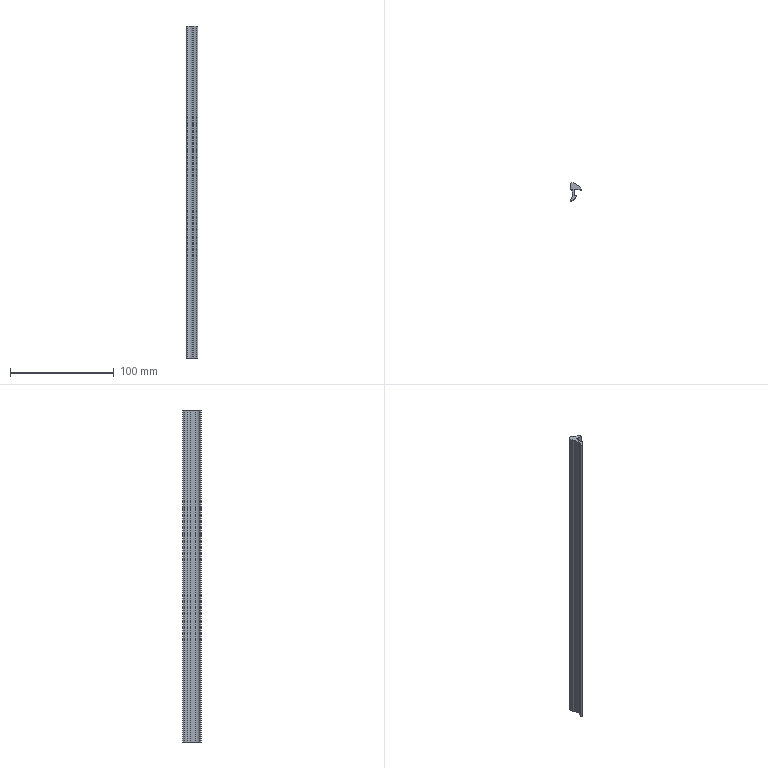Part | SolidWorks | features BaseBody 1, MoveFace 1 | 1 solid | 20 faces | box 10.8 x 17.5 x 320 mm | volume 25216 mm3 | cylinder 11 | plane 9 | commonest cylinder face diameters 1.6 x2 14 x2 0.4 x1 0.6 x1 0.8 x1 2.6 x1
STEP:
#1=CARTESIAN_POINT('',(-3.236,-11.055,220.));
#2=VERTEX_POINT('',#1);
#3=CARTESIAN_POINT('',(-4.3,-10.3,220.));
#4=VERTEX_POINT('',#3);
#5=CARTESIAN_POINT('',(-3.5,-10.3,220.));
#6=DIRECTION('',(0.,0.,-1.));
#7=DIRECTION('',(1.,0.,0.));
#8=AXIS2_PLACEMENT_3D('',#5,#6,#7);
#9=CIRCLE('',#8,0.8);
#10=EDGE_CURVE('',#2,#4,#9,.T.);
#11=ORIENTED_EDGE('',*,*,#10,.T.);
#12=CARTESIAN_POINT('',(-4.3,-10.3,-100.));
#13=VERTEX_POINT('',#12);
#14=CARTESIAN_POINT('',(-4.3,-10.3,-100.));
#15=DIRECTION('',(0.,0.,-1.));
#16=VECTOR('',#15,1000.);
#17=LINE('',#14,#16);
#18=EDGE_CURVE('',#4,#13,#17,.T.);
#19=ORIENTED_EDGE('',*,*,#18,.T.);
#20=CARTESIAN_POINT('',(-3.236,-11.055,-100.));
#21=VERTEX_POINT('',#20);
#22=CARTESIAN_POINT('',(-3.5,-10.3,-100.));
#23=DIRECTION('',(0.,0.,1.));
#24=DIRECTION('',(-1.,0.,0.));
#25=AXIS2_PLACEMENT_3D('',#22,#23,#24);
#26=CIRCLE('',#25,0.8);
#27=EDGE_CURVE('',#13,#21,#26,.T.);
#28=ORIENTED_EDGE('',*,*,#27,.T.);
#29=CARTESIAN_POINT('',(-3.236,-11.055,-100.));
#30=DIRECTION('',(0.,0.,-1.));
#31=VECTOR('',#30,1000.);
#32=LINE('',#29,#31);
#33=EDGE_CURVE('',#2,#21,#32,.T.);
#34=ORIENTED_EDGE('',*,*,#33,.F.);
#35=EDGE_LOOP('',(#11,#19,#28,#34));
#36=FACE_OUTER_BOUND('',#35,.T.);
#37=CARTESIAN_POINT('',(-3.5,-10.3,-100.));
#38=DIRECTION('',(0.,0.,-1.));
#39=DIRECTION('',(-1.,0.,0.));
#40=AXIS2_PLACEMENT_3D('',#37,#38,#39);
#41=CYLINDRICAL_SURFACE('',#40,0.8);
#42=ADVANCED_FACE('',(#36),#41,.T.);
#43=CARTESIAN_POINT('',(1.184,-6.397,-100.));
#44=VERTEX_POINT('',#43);
#45=CARTESIAN_POINT('',(-5.702,-4.29,-100.));
#46=DIRECTION('',(0.,0.,1.));
#47=DIRECTION('',(-1.,0.,0.));
#48=AXIS2_PLACEMENT_3D('',#45,#46,#47);
#49=CIRCLE('',#48,7.201);
#50=EDGE_CURVE('',#21,#44,#49,.T.);
#51=ORIENTED_EDGE('',*,*,#50,.T.);
#52=CARTESIAN_POINT('',(1.184,-6.397,220.));
#53=VERTEX_POINT('',#52);
#54=CARTESIAN_POINT('',(1.184,-6.397,-100.));
#55=DIRECTION('',(0.,0.,1.));
#56=VECTOR('',#55,1000.);
#57=LINE('',#54,#56);
#58=EDGE_CURVE('',#44,#53,#57,.T.);
#59=ORIENTED_EDGE('',*,*,#58,.T.);
#60=CARTESIAN_POINT('',(-5.702,-4.29,220.));
#61=DIRECTION('',(0.,0.,-1.));
#62=DIRECTION('',(1.,0.,0.));
#63=AXIS2_PLACEMENT_3D('',#60,#61,#62);
#64=CIRCLE('',#63,7.201);
#65=EDGE_CURVE('',#53,#2,#64,.T.);
#66=ORIENTED_EDGE('',*,*,#65,.T.);
#67=ORIENTED_EDGE('',*,*,#33,.T.);
#68=EDGE_LOOP('',(#51,#59,#66,#67));
#69=FACE_OUTER_BOUND('',#68,.T.);
#70=CARTESIAN_POINT('',(-5.702,-4.29,-100.));
#71=DIRECTION('',(0.,0.,-1.));
#72=DIRECTION('',(-1.,0.,0.));
#73=AXIS2_PLACEMENT_3D('',#70,#71,#72);
#74=CYLINDRICAL_SURFACE('',#73,7.201);
#75=ADVANCED_FACE('',(#69),#74,.T.);
#76=CARTESIAN_POINT('',(0.9,-6.,-100.));
#77=VERTEX_POINT('',#76);
#78=CARTESIAN_POINT('',(0.9,-6.3,-100.));
#79=DIRECTION('',(0.,0.,1.));
#80=DIRECTION('',(-1.,0.,0.));
#81=AXIS2_PLACEMENT_3D('',#78,#79,#80);
#82=CIRCLE('',#81,0.3);
#83=EDGE_CURVE('',#44,#77,#82,.T.);
#84=ORIENTED_EDGE('',*,*,#83,.T.);
#85=CARTESIAN_POINT('',(0.9,-6.,220.));
#86=VERTEX_POINT('',#85);
#87=CARTESIAN_POINT('',(0.9,-6.,-100.));
#88=DIRECTION('',(0.,0.,1.));
#89=VECTOR('',#88,1000.);
#90=LINE('',#87,#89);
#91=EDGE_CURVE('',#77,#86,#90,.T.);
#92=ORIENTED_EDGE('',*,*,#91,.T.);
#93=CARTESIAN_POINT('',(0.9,-6.3,220.));
#94=DIRECTION('',(0.,0.,-1.));
#95=DIRECTION('',(1.,0.,0.));
#96=AXIS2_PLACEMENT_3D('',#93,#94,#95);
#97=CIRCLE('',#96,0.3);
#98=EDGE_CURVE('',#86,#53,#97,.T.);
#99=ORIENTED_EDGE('',*,*,#98,.T.);
#100=ORIENTED_EDGE('',*,*,#58,.F.);
#101=EDGE_LOOP('',(#84,#92,#99,#100));
#102=FACE_OUTER_BOUND('',#101,.T.);
#103=CARTESIAN_POINT('',(0.9,-6.3,-100.));
#104=DIRECTION('',(0.,0.,-1.));
#105=DIRECTION('',(-1.,0.,0.));
#106=AXIS2_PLACEMENT_3D('',#103,#104,#105);
#107=CYLINDRICAL_SURFACE('',#106,0.3);
#108=ADVANCED_FACE('',(#102),#107,.T.);
#109=CARTESIAN_POINT('',(-2.5,-0.5,-100.));
#110=VERTEX_POINT('',#109);
#111=CARTESIAN_POINT('',(-2.5,-6.153,-100.));
#112=VERTEX_POINT('',#111);
#113=CARTESIAN_POINT('',(-2.5,-6.397,-100.));
#114=DIRECTION('',(0.,-1.,0.));
#115=VECTOR('',#114,1000.);
#116=LINE('',#113,#115);
#117=EDGE_CURVE('',#110,#112,#116,.T.);
#118=ORIENTED_EDGE('',*,*,#117,.F.);
#119=CARTESIAN_POINT('',(-4.2,1.695,-100.));
#120=VERTEX_POINT('',#119);
#121=CARTESIAN_POINT('',(-1.701,1.875,-100.));
#122=DIRECTION('',(0.,0.,1.));
#123=DIRECTION('',(-1.,0.,0.));
#124=AXIS2_PLACEMENT_3D('',#121,#122,#123);
#125=CIRCLE('',#124,2.506);
#126=EDGE_CURVE('',#120,#110,#125,.T.);
#127=ORIENTED_EDGE('',*,*,#126,.F.);
#128=CARTESIAN_POINT('',(-4.2,5.1,-100.));
#129=VERTEX_POINT('',#128);
#130=CARTESIAN_POINT('',(-4.2,-6.397,-100.));
#131=DIRECTION('',(0.,-1.,0.));
#132=VECTOR('',#131,1000.);
#133=LINE('',#130,#132);
#134=EDGE_CURVE('',#129,#120,#133,.T.);
#135=ORIENTED_EDGE('',*,*,#134,.F.);
#136=CARTESIAN_POINT('',(-2.892,6.4,-100.));
#137=VERTEX_POINT('',#136);
#138=CARTESIAN_POINT('',(-2.9,5.1,-100.));
#139=DIRECTION('',(0.,0.,1.));
#140=DIRECTION('',(-1.,0.,0.));
#141=AXIS2_PLACEMENT_3D('',#138,#139,#140);
#142=CIRCLE('',#141,1.3);
#143=EDGE_CURVE('',#137,#129,#142,.T.);
#144=ORIENTED_EDGE('',*,*,#143,.F.);
#145=CARTESIAN_POINT('',(0.5,5.5,-100.));
#146=VERTEX_POINT('',#145);
#147=CARTESIAN_POINT('',(-2.934,-0.5999,-100.));
#148=DIRECTION('',(0.,0.,1.));
#149=DIRECTION('',(-1.,0.,0.));
#150=AXIS2_PLACEMENT_3D('',#147,#148,#149);
#151=CIRCLE('',#150,7.);
#152=EDGE_CURVE('',#146,#137,#151,.T.);
#153=ORIENTED_EDGE('',*,*,#152,.F.);
#154=CARTESIAN_POINT('',(5.5,1.7,-100.));
#155=VERTEX_POINT('',#154);
#156=CARTESIAN_POINT('',(5.5,1.7,-100.));
#157=DIRECTION('',(-0.7962,0.6051,0.));
#158=VECTOR('',#157,1000.);
#159=LINE('',#156,#158);
#160=EDGE_CURVE('',#155,#146,#159,.T.);
#161=ORIENTED_EDGE('',*,*,#160,.F.);
#162=CARTESIAN_POINT('',(6.458,-0.2215,-100.));
#163=VERTEX_POINT('',#162);
#164=CARTESIAN_POINT('',(6.458,-0.2215,-100.));
#165=DIRECTION('',(-0.4462,0.8949,0.));
#166=VECTOR('',#165,1000.);
#167=LINE('',#164,#166);
#168=EDGE_CURVE('',#163,#155,#167,.T.);
#169=ORIENTED_EDGE('',*,*,#168,.F.);
#170=CARTESIAN_POINT('',(5.895,-0.7433,-100.));
#171=VERTEX_POINT('',#170);
#172=CARTESIAN_POINT('',(6.1,-0.4,-100.));
#173=DIRECTION('',(0.,0.,1.));
#174=DIRECTION('',(-1.,0.,0.));
#175=AXIS2_PLACEMENT_3D('',#172,#173,#174);
#176=CIRCLE('',#175,0.4);
#177=EDGE_CURVE('',#171,#163,#176,.T.);
#178=ORIENTED_EDGE('',*,*,#177,.F.);
#179=CARTESIAN_POINT('',(3.,0.,-100.));
#180=VERTEX_POINT('',#179);
#181=CARTESIAN_POINT('',(2.746,-6.995,-100.));
#182=DIRECTION('',(0.,0.,-1.));
#183=DIRECTION('',(-1.,0.,0.));
#184=AXIS2_PLACEMENT_3D('',#181,#182,#183);
#185=CIRCLE('',#184,7.);
#186=EDGE_CURVE('',#180,#171,#185,.T.);
#187=ORIENTED_EDGE('',*,*,#186,.F.);
#188=CARTESIAN_POINT('',(0.,0.,-100.));
#189=VERTEX_POINT('',#188);
#190=CARTESIAN_POINT('',(-6.814,0.,-100.));
#191=DIRECTION('',(1.,0.,0.));
#192=VECTOR('',#191,1000.);
#193=LINE('',#190,#192);
#194=EDGE_CURVE('',#189,#180,#193,.T.);
#195=ORIENTED_EDGE('',*,*,#194,.F.);
#196=CARTESIAN_POINT('',(0.,-5.8,-100.));
#197=VERTEX_POINT('',#196);
#198=CARTESIAN_POINT('',(0.,-6.397,-100.));
#199=DIRECTION('',(0.,1.,0.));
#200=VECTOR('',#199,1000.);
#201=LINE('',#198,#200);
#202=EDGE_CURVE('',#197,#189,#201,.T.);
#203=ORIENTED_EDGE('',*,*,#202,.F.);
#204=CARTESIAN_POINT('',(0.2,-6.,-100.));
#205=VERTEX_POINT('',#204);
#206=CARTESIAN_POINT('',(0.2,-5.8,-100.));
#207=DIRECTION('',(0.,0.,1.));
#208=DIRECTION('',(-1.,0.,0.));
#209=AXIS2_PLACEMENT_3D('',#206,#207,#208);
#210=CIRCLE('',#209,0.2);
#211=EDGE_CURVE('',#197,#205,#210,.T.);
#212=ORIENTED_EDGE('',*,*,#211,.T.);
#213=CARTESIAN_POINT('',(-6.814,-6.,-100.));
#214=DIRECTION('',(-1.,0.,0.));
#215=VECTOR('',#214,1000.);
#216=LINE('',#213,#215);
#217=EDGE_CURVE('',#77,#205,#216,.T.);
#218=ORIENTED_EDGE('',*,*,#217,.F.);
#219=ORIENTED_EDGE('',*,*,#83,.F.);
#220=ORIENTED_EDGE('',*,*,#50,.F.);
#221=ORIENTED_EDGE('',*,*,#27,.F.);
#222=CARTESIAN_POINT('',(-3.998,-9.674,-100.));
#223=VERTEX_POINT('',#222);
#224=CARTESIAN_POINT('',(-3.5,-10.3,-100.));
#225=DIRECTION('',(0.,0.,1.));
#226=DIRECTION('',(-1.,0.,0.));
#227=AXIS2_PLACEMENT_3D('',#224,#225,#226);
#228=CIRCLE('',#227,0.8);
#229=EDGE_CURVE('',#223,#13,#228,.T.);
#230=ORIENTED_EDGE('',*,*,#229,.F.);
#231=CARTESIAN_POINT('',(-6.814,-6.397,-100.));
#232=DIRECTION('',(0.,0.,-1.));
#233=DIRECTION('',(-1.,0.,0.));
#234=AXIS2_PLACEMENT_3D('',#231,#232,#233);
#235=CIRCLE('',#234,4.321);
#236=EDGE_CURVE('',#112,#223,#235,.T.);
#237=ORIENTED_EDGE('',*,*,#236,.F.);
#238=EDGE_LOOP('',(#118,#127,#135,#144,#153,#161,#169,#178,#187,#195,#203,#212,#218,#219,#220,#221,#230,#237));
#239=FACE_OUTER_BOUND('',#238,.T.);
#240=CARTESIAN_POINT('',(-6.814,-6.397,-100.));
#241=DIRECTION('',(0.,0.,1.));
#242=DIRECTION('',(1.,0.,0.));
#243=AXIS2_PLACEMENT_3D('',#240,#241,#242);
#244=PLANE('',#243);
#245=ADVANCED_FACE('',(#239),#244,.F.);
#246=ORIENTED_EDGE('',*,*,#18,.F.);
#247=CARTESIAN_POINT('',(-3.998,-9.674,220.));
#248=VERTEX_POINT('',#247);
#249=CARTESIAN_POINT('',(-3.5,-10.3,220.));
#250=DIRECTION('',(0.,0.,-1.));
#251=DIRECTION('',(1.,0.,0.));
#252=AXIS2_PLACEMENT_3D('',#249,#250,#251);
#253=CIRCLE('',#252,0.8);
#254=EDGE_CURVE('',#4,#248,#253,.T.);
#255=ORIENTED_EDGE('',*,*,#254,.T.);
#256=CARTESIAN_POINT('',(-3.998,-9.674,-100.));
#257=DIRECTION('',(0.,0.,-1.));
#258=VECTOR('',#257,1000.);
#259=LINE('',#256,#258);
#260=EDGE_CURVE('',#248,#223,#259,.T.);
#261=ORIENTED_EDGE('',*,*,#260,.T.);
#262=ORIENTED_EDGE('',*,*,#229,.T.);
#263=EDGE_LOOP('',(#246,#255,#261,#262));
#264=FACE_OUTER_BOUND('',#263,.T.);
#265=CARTESIAN_POINT('',(-3.5,-10.3,-100.));
#266=DIRECTION('',(0.,0.,-1.));
#267=DIRECTION('',(-1.,0.,0.));
#268=AXIS2_PLACEMENT_3D('',#265,#266,#267);
#269=CYLINDRICAL_SURFACE('',#268,0.8);
#270=ADVANCED_FACE('',(#264),#269,.T.);
#271=CARTESIAN_POINT('',(-4.2,1.695,220.));
#272=VERTEX_POINT('',#271);
#273=CARTESIAN_POINT('',(-2.5,-0.5,220.));
#274=VERTEX_POINT('',#273);
#275=CARTESIAN_POINT('',(-1.701,1.875,220.));
#276=DIRECTION('',(0.,0.,1.));
#277=DIRECTION('',(1.,0.,0.));
#278=AXIS2_PLACEMENT_3D('',#275,#276,#277);
#279=CIRCLE('',#278,2.506);
#280=EDGE_CURVE('',#272,#274,#279,.T.);
#281=ORIENTED_EDGE('',*,*,#280,.T.);
#282=CARTESIAN_POINT('',(-2.5,-6.153,220.));
#283=VERTEX_POINT('',#282);
#284=CARTESIAN_POINT('',(-2.5,-6.397,220.));
#285=DIRECTION('',(0.,-1.,0.));
#286=VECTOR('',#285,1000.);
#287=LINE('',#284,#286);
#288=EDGE_CURVE('',#274,#283,#287,.T.);
#289=ORIENTED_EDGE('',*,*,#288,.T.);
#290=CARTESIAN_POINT('',(-6.814,-6.397,220.));
#291=DIRECTION('',(0.,0.,-1.));
#292=DIRECTION('',(1.,0.,0.));
#293=AXIS2_PLACEMENT_3D('',#290,#291,#292);
#294=CIRCLE('',#293,4.321);
#295=EDGE_CURVE('',#283,#248,#294,.T.);
#296=ORIENTED_EDGE('',*,*,#295,.T.);
#297=ORIENTED_EDGE('',*,*,#254,.F.);
#298=ORIENTED_EDGE('',*,*,#10,.F.);
#299=ORIENTED_EDGE('',*,*,#65,.F.);
#300=ORIENTED_EDGE('',*,*,#98,.F.);
#301=CARTESIAN_POINT('',(0.2,-6.,220.));
#302=VERTEX_POINT('',#301);
#303=CARTESIAN_POINT('',(-6.814,-6.,220.));
#304=DIRECTION('',(-1.,0.,0.));
#305=VECTOR('',#304,1000.);
#306=LINE('',#303,#305);
#307=EDGE_CURVE('',#86,#302,#306,.T.);
#308=ORIENTED_EDGE('',*,*,#307,.T.);
#309=CARTESIAN_POINT('',(0.,-5.8,220.));
#310=VERTEX_POINT('',#309);
#311=CARTESIAN_POINT('',(0.2,-5.8,220.));
#312=DIRECTION('',(0.,0.,-1.));
#313=DIRECTION('',(1.,0.,0.));
#314=AXIS2_PLACEMENT_3D('',#311,#312,#313);
#315=CIRCLE('',#314,0.2);
#316=EDGE_CURVE('',#302,#310,#315,.T.);
#317=ORIENTED_EDGE('',*,*,#316,.T.);
#318=CARTESIAN_POINT('',(0.,0.,220.));
#319=VERTEX_POINT('',#318);
#320=CARTESIAN_POINT('',(0.,-6.397,220.));
#321=DIRECTION('',(0.,1.,0.));
#322=VECTOR('',#321,1000.);
#323=LINE('',#320,#322);
#324=EDGE_CURVE('',#310,#319,#323,.T.);
#325=ORIENTED_EDGE('',*,*,#324,.T.);
#326=CARTESIAN_POINT('',(3.,0.,220.));
#327=VERTEX_POINT('',#326);
#328=CARTESIAN_POINT('',(-6.814,0.,220.));
#329=DIRECTION('',(1.,0.,0.));
#330=VECTOR('',#329,1000.);
#331=LINE('',#328,#330);
#332=EDGE_CURVE('',#319,#327,#331,.T.);
#333=ORIENTED_EDGE('',*,*,#332,.T.);
#334=CARTESIAN_POINT('',(5.895,-0.7433,220.));
#335=VERTEX_POINT('',#334);
#336=CARTESIAN_POINT('',(2.746,-6.995,220.));
#337=DIRECTION('',(0.,0.,-1.));
#338=DIRECTION('',(1.,0.,0.));
#339=AXIS2_PLACEMENT_3D('',#336,#337,#338);
#340=CIRCLE('',#339,7.);
#341=EDGE_CURVE('',#327,#335,#340,.T.);
#342=ORIENTED_EDGE('',*,*,#341,.T.);
#343=CARTESIAN_POINT('',(6.458,-0.2215,220.));
#344=VERTEX_POINT('',#343);
#345=CARTESIAN_POINT('',(6.1,-0.4,220.));
#346=DIRECTION('',(0.,0.,-1.));
#347=DIRECTION('',(1.,0.,0.));
#348=AXIS2_PLACEMENT_3D('',#345,#346,#347);
#349=CIRCLE('',#348,0.4);
#350=EDGE_CURVE('',#344,#335,#349,.T.);
#351=ORIENTED_EDGE('',*,*,#350,.F.);
#352=CARTESIAN_POINT('',(5.5,1.7,220.));
#353=VERTEX_POINT('',#352);
#354=CARTESIAN_POINT('',(6.282,0.1323,220.));
#355=DIRECTION('',(-0.4462,0.8949,0.));
#356=VECTOR('',#355,1000.);
#357=LINE('',#354,#356);
#358=EDGE_CURVE('',#344,#353,#357,.T.);
#359=ORIENTED_EDGE('',*,*,#358,.T.);
#360=CARTESIAN_POINT('',(0.5,5.5,220.));
#361=VERTEX_POINT('',#360);
#362=CARTESIAN_POINT('',(1.595,4.668,220.));
#363=DIRECTION('',(-0.7962,0.6051,0.));
#364=VECTOR('',#363,1000.);
#365=LINE('',#362,#364);
#366=EDGE_CURVE('',#353,#361,#365,.T.);
#367=ORIENTED_EDGE('',*,*,#366,.T.);
#368=CARTESIAN_POINT('',(-2.892,6.4,220.));
#369=VERTEX_POINT('',#368);
#370=CARTESIAN_POINT('',(-2.934,-0.5999,220.));
#371=DIRECTION('',(0.,0.,1.));
#372=DIRECTION('',(1.,0.,0.));
#373=AXIS2_PLACEMENT_3D('',#370,#371,#372);
#374=CIRCLE('',#373,7.);
#375=EDGE_CURVE('',#361,#369,#374,.T.);
#376=ORIENTED_EDGE('',*,*,#375,.T.);
#377=CARTESIAN_POINT('',(-4.2,5.1,220.));
#378=VERTEX_POINT('',#377);
#379=CARTESIAN_POINT('',(-2.9,5.1,220.));
#380=DIRECTION('',(0.,0.,1.));
#381=DIRECTION('',(1.,0.,0.));
#382=AXIS2_PLACEMENT_3D('',#379,#380,#381);
#383=CIRCLE('',#382,1.3);
#384=EDGE_CURVE('',#369,#378,#383,.T.);
#385=ORIENTED_EDGE('',*,*,#384,.T.);
#386=CARTESIAN_POINT('',(-4.2,-6.397,220.));
#387=DIRECTION('',(0.,-1.,0.));
#388=VECTOR('',#387,1000.);
#389=LINE('',#386,#388);
#390=EDGE_CURVE('',#378,#272,#389,.T.);
#391=ORIENTED_EDGE('',*,*,#390,.T.);
#392=EDGE_LOOP('',(#281,#289,#296,#297,#298,#299,#300,#308,#317,#325,#333,#342,#351,#359,#367,#376,#385,#391));
#393=FACE_OUTER_BOUND('',#392,.T.);
#394=CARTESIAN_POINT('',(-6.814,-6.397,220.));
#395=DIRECTION('',(0.,0.,1.));
#396=DIRECTION('',(1.,0.,0.));
#397=AXIS2_PLACEMENT_3D('',#394,#395,#396);
#398=PLANE('',#397);
#399=ADVANCED_FACE('',(#393),#398,.T.);
#400=ORIENTED_EDGE('',*,*,#217,.T.);
#401=CARTESIAN_POINT('',(0.2,-6.,-100.));
#402=DIRECTION('',(0.,0.,1.));
#403=VECTOR('',#402,1000.);
#404=LINE('',#401,#403);
#405=EDGE_CURVE('',#205,#302,#404,.T.);
#406=ORIENTED_EDGE('',*,*,#405,.T.);
#407=ORIENTED_EDGE('',*,*,#307,.F.);
#408=ORIENTED_EDGE('',*,*,#91,.F.);
#409=EDGE_LOOP('',(#400,#406,#407,#408));
#410=FACE_OUTER_BOUND('',#409,.T.);
#411=CARTESIAN_POINT('',(0.9,-6.,-100.));
#412=DIRECTION('',(0.,1.,0.));
#413=DIRECTION('',(0.,0.,1.));
#414=AXIS2_PLACEMENT_3D('',#411,#412,#413);
#415=PLANE('',#414);
#416=ADVANCED_FACE('',(#410),#415,.T.);
#417=CARTESIAN_POINT('',(-2.5,-6.153,-100.));
#418=DIRECTION('',(0.,0.,1.));
#419=VECTOR('',#418,1000.);
#420=LINE('',#417,#419);
#421=EDGE_CURVE('',#112,#283,#420,.T.);
#422=ORIENTED_EDGE('',*,*,#421,.F.);
#423=ORIENTED_EDGE('',*,*,#236,.T.);
#424=ORIENTED_EDGE('',*,*,#260,.F.);
#425=ORIENTED_EDGE('',*,*,#295,.F.);
#426=EDGE_LOOP('',(#422,#423,#424,#425));
#427=FACE_OUTER_BOUND('',#426,.T.);
#428=CARTESIAN_POINT('',(-6.814,-6.397,-100.));
#429=DIRECTION('',(0.,0.,-1.));
#430=DIRECTION('',(-1.,0.,0.));
#431=AXIS2_PLACEMENT_3D('',#428,#429,#430);
#432=CYLINDRICAL_SURFACE('',#431,4.321);
#433=ADVANCED_FACE('',(#427),#432,.F.);
#434=ORIENTED_EDGE('',*,*,#117,.T.);
#435=ORIENTED_EDGE('',*,*,#421,.T.);
#436=ORIENTED_EDGE('',*,*,#288,.F.);
#437=CARTESIAN_POINT('',(-2.5,-0.5,-100.));
#438=DIRECTION('',(0.,0.,-1.));
#439=VECTOR('',#438,1000.);
#440=LINE('',#437,#439);
#441=EDGE_CURVE('',#274,#110,#440,.T.);
#442=ORIENTED_EDGE('',*,*,#441,.T.);
#443=EDGE_LOOP('',(#434,#435,#436,#442));
#444=FACE_OUTER_BOUND('',#443,.T.);
#445=CARTESIAN_POINT('',(-2.5,-0.5,-100.));
#446=DIRECTION('',(-1.,0.,0.));
#447=DIRECTION('',(0.,0.,1.));
#448=AXIS2_PLACEMENT_3D('',#445,#446,#447);
#449=PLANE('',#448);
#450=ADVANCED_FACE('',(#444),#449,.T.);
#451=ORIENTED_EDGE('',*,*,#126,.T.);
#452=ORIENTED_EDGE('',*,*,#441,.F.);
#453=ORIENTED_EDGE('',*,*,#280,.F.);
#454=CARTESIAN_POINT('',(-4.2,1.695,-100.));
#455=DIRECTION('',(0.,0.,-1.));
#456=VECTOR('',#455,1000.);
#457=LINE('',#454,#456);
#458=EDGE_CURVE('',#272,#120,#457,.T.);
#459=ORIENTED_EDGE('',*,*,#458,.T.);
#460=EDGE_LOOP('',(#451,#452,#453,#459));
#461=FACE_OUTER_BOUND('',#460,.T.);
#462=CARTESIAN_POINT('',(-1.701,1.875,-100.));
#463=DIRECTION('',(0.,0.,-1.));
#464=DIRECTION('',(-1.,0.,0.));
#465=AXIS2_PLACEMENT_3D('',#462,#463,#464);
#466=CYLINDRICAL_SURFACE('',#465,2.506);
#467=ADVANCED_FACE('',(#461),#466,.T.);
#468=ORIENTED_EDGE('',*,*,#134,.T.);
#469=ORIENTED_EDGE('',*,*,#458,.F.);
#470=ORIENTED_EDGE('',*,*,#390,.F.);
#471=CARTESIAN_POINT('',(-4.2,5.1,-100.));
#472=DIRECTION('',(0.,0.,-1.));
#473=VECTOR('',#472,1000.);
#474=LINE('',#471,#473);
#475=EDGE_CURVE('',#378,#129,#474,.T.);
#476=ORIENTED_EDGE('',*,*,#475,.T.);
#477=EDGE_LOOP('',(#468,#469,#470,#476));
#478=FACE_OUTER_BOUND('',#477,.T.);
#479=CARTESIAN_POINT('',(-4.2,5.1,-100.));
#480=DIRECTION('',(-1.,0.,0.));
#481=DIRECTION('',(0.,0.,1.));
#482=AXIS2_PLACEMENT_3D('',#479,#480,#481);
#483=PLANE('',#482);
#484=ADVANCED_FACE('',(#478),#483,.T.);
#485=ORIENTED_EDGE('',*,*,#143,.T.);
#486=ORIENTED_EDGE('',*,*,#475,.F.);
#487=ORIENTED_EDGE('',*,*,#384,.F.);
#488=CARTESIAN_POINT('',(-2.892,6.4,-100.));
#489=DIRECTION('',(0.,0.,-1.));
#490=VECTOR('',#489,1000.);
#491=LINE('',#488,#490);
#492=EDGE_CURVE('',#369,#137,#491,.T.);
#493=ORIENTED_EDGE('',*,*,#492,.T.);
#494=EDGE_LOOP('',(#485,#486,#487,#493));
#495=FACE_OUTER_BOUND('',#494,.T.);
#496=CARTESIAN_POINT('',(-2.9,5.1,-100.));
#497=DIRECTION('',(0.,0.,-1.));
#498=DIRECTION('',(-1.,0.,0.));
#499=AXIS2_PLACEMENT_3D('',#496,#497,#498);
#500=CYLINDRICAL_SURFACE('',#499,1.3);
#501=ADVANCED_FACE('',(#495),#500,.T.);
#502=ORIENTED_EDGE('',*,*,#152,.T.);
#503=ORIENTED_EDGE('',*,*,#492,.F.);
#504=ORIENTED_EDGE('',*,*,#375,.F.);
#505=CARTESIAN_POINT('',(0.5,5.5,-100.));
#506=DIRECTION('',(0.,0.,-1.));
#507=VECTOR('',#506,1000.);
#508=LINE('',#505,#507);
#509=EDGE_CURVE('',#361,#146,#508,.T.);
#510=ORIENTED_EDGE('',*,*,#509,.T.);
#511=EDGE_LOOP('',(#502,#503,#504,#510));
#512=FACE_OUTER_BOUND('',#511,.T.);
#513=CARTESIAN_POINT('',(-2.934,-0.5999,-100.));
#514=DIRECTION('',(0.,0.,-1.));
#515=DIRECTION('',(-1.,0.,0.));
#516=AXIS2_PLACEMENT_3D('',#513,#514,#515);
#517=CYLINDRICAL_SURFACE('',#516,7.);
#518=ADVANCED_FACE('',(#512),#517,.T.);
#519=ORIENTED_EDGE('',*,*,#160,.T.);
#520=ORIENTED_EDGE('',*,*,#509,.F.);
#521=ORIENTED_EDGE('',*,*,#366,.F.);
#522=CARTESIAN_POINT('',(5.5,1.7,-100.));
#523=DIRECTION('',(0.,0.,-1.));
#524=VECTOR('',#523,1000.);
#525=LINE('',#522,#524);
#526=EDGE_CURVE('',#353,#155,#525,.T.);
#527=ORIENTED_EDGE('',*,*,#526,.T.);
#528=EDGE_LOOP('',(#519,#520,#521,#527));
#529=FACE_OUTER_BOUND('',#528,.T.);
#530=CARTESIAN_POINT('',(5.5,1.7,-100.));
#531=DIRECTION('',(0.6051,0.7962,0.));
#532=DIRECTION('',(-0.7962,0.6051,0.));
#533=AXIS2_PLACEMENT_3D('',#530,#531,#532);
#534=PLANE('',#533);
#535=ADVANCED_FACE('',(#529),#534,.T.);
#536=ORIENTED_EDGE('',*,*,#168,.T.);
#537=ORIENTED_EDGE('',*,*,#526,.F.);
#538=ORIENTED_EDGE('',*,*,#358,.F.);
#539=CARTESIAN_POINT('',(6.458,-0.2215,-100.));
#540=DIRECTION('',(0.,0.,-1.));
#541=VECTOR('',#540,1000.);
#542=LINE('',#539,#541);
#543=EDGE_CURVE('',#344,#163,#542,.T.);
#544=ORIENTED_EDGE('',*,*,#543,.T.);
#545=EDGE_LOOP('',(#536,#537,#538,#544));
#546=FACE_OUTER_BOUND('',#545,.T.);
#547=CARTESIAN_POINT('',(6.458,-0.2215,-100.));
#548=DIRECTION('',(0.8949,0.4462,0.));
#549=DIRECTION('',(-0.4462,0.8949,0.));
#550=AXIS2_PLACEMENT_3D('',#547,#548,#549);
#551=PLANE('',#550);
#552=ADVANCED_FACE('',(#546),#551,.T.);
#553=CARTESIAN_POINT('',(3.,0.,-100.));
#554=DIRECTION('',(0.,0.,1.));
#555=VECTOR('',#554,1000.);
#556=LINE('',#553,#555);
#557=EDGE_CURVE('',#180,#327,#556,.T.);
#558=ORIENTED_EDGE('',*,*,#557,.F.);
#559=ORIENTED_EDGE('',*,*,#186,.T.);
#560=CARTESIAN_POINT('',(5.895,-0.7433,-100.));
#561=DIRECTION('',(0.,0.,-1.));
#562=VECTOR('',#561,1000.);
#563=LINE('',#560,#562);
#564=EDGE_CURVE('',#335,#171,#563,.T.);
#565=ORIENTED_EDGE('',*,*,#564,.F.);
#566=ORIENTED_EDGE('',*,*,#341,.F.);
#567=EDGE_LOOP('',(#558,#559,#565,#566));
#568=FACE_OUTER_BOUND('',#567,.T.);
#569=CARTESIAN_POINT('',(2.746,-6.995,-100.));
#570=DIRECTION('',(0.,0.,-1.));
#571=DIRECTION('',(-1.,0.,0.));
#572=AXIS2_PLACEMENT_3D('',#569,#570,#571);
#573=CYLINDRICAL_SURFACE('',#572,7.);
#574=ADVANCED_FACE('',(#568),#573,.F.);
#575=ORIENTED_EDGE('',*,*,#194,.T.);
#576=ORIENTED_EDGE('',*,*,#557,.T.);
#577=ORIENTED_EDGE('',*,*,#332,.F.);
#578=CARTESIAN_POINT('',(0.,0.,-100.));
#579=DIRECTION('',(0.,0.,-1.));
#580=VECTOR('',#579,1000.);
#581=LINE('',#578,#580);
#582=EDGE_CURVE('',#319,#189,#581,.T.);
#583=ORIENTED_EDGE('',*,*,#582,.T.);
#584=EDGE_LOOP('',(#575,#576,#577,#583));
#585=FACE_OUTER_BOUND('',#584,.T.);
#586=CARTESIAN_POINT('',(0.,0.,-100.));
#587=DIRECTION('',(0.,-1.,0.));
#588=DIRECTION('',(0.,0.,-1.));
#589=AXIS2_PLACEMENT_3D('',#586,#587,#588);
#590=PLANE('',#589);
#591=ADVANCED_FACE('',(#585),#590,.T.);
#592=ORIENTED_EDGE('',*,*,#202,.T.);
#593=ORIENTED_EDGE('',*,*,#582,.F.);
#594=ORIENTED_EDGE('',*,*,#324,.F.);
#595=CARTESIAN_POINT('',(0.,-5.8,-100.));
#596=DIRECTION('',(0.,0.,-1.));
#597=VECTOR('',#596,1000.);
#598=LINE('',#595,#597);
#599=EDGE_CURVE('',#310,#197,#598,.T.);
#600=ORIENTED_EDGE('',*,*,#599,.T.);
#601=EDGE_LOOP('',(#592,#593,#594,#600));
#602=FACE_OUTER_BOUND('',#601,.T.);
#603=CARTESIAN_POINT('',(0.,-5.8,-100.));
#604=DIRECTION('',(1.,0.,0.));
#605=DIRECTION('',(0.,0.,-1.));
#606=AXIS2_PLACEMENT_3D('',#603,#604,#605);
#607=PLANE('',#606);
#608=ADVANCED_FACE('',(#602),#607,.T.);
#609=ORIENTED_EDGE('',*,*,#405,.F.);
#610=ORIENTED_EDGE('',*,*,#211,.F.);
#611=ORIENTED_EDGE('',*,*,#599,.F.);
#612=ORIENTED_EDGE('',*,*,#316,.F.);
#613=EDGE_LOOP('',(#609,#610,#611,#612));
#614=FACE_OUTER_BOUND('',#613,.T.);
#615=CARTESIAN_POINT('',(0.2,-5.8,-100.));
#616=DIRECTION('',(0.,0.,-1.));
#617=DIRECTION('',(-1.,0.,0.));
#618=AXIS2_PLACEMENT_3D('',#615,#616,#617);
#619=CYLINDRICAL_SURFACE('',#618,0.2);
#620=ADVANCED_FACE('',(#614),#619,.F.);
#621=ORIENTED_EDGE('',*,*,#177,.T.);
#622=ORIENTED_EDGE('',*,*,#543,.F.);
#623=ORIENTED_EDGE('',*,*,#350,.T.);
#624=ORIENTED_EDGE('',*,*,#564,.T.);
#625=EDGE_LOOP('',(#621,#622,#623,#624));
#626=FACE_OUTER_BOUND('',#625,.T.);
#627=CARTESIAN_POINT('',(6.1,-0.4,-100.));
#628=DIRECTION('',(0.,0.,-1.));
#629=DIRECTION('',(-1.,0.,0.));
#630=AXIS2_PLACEMENT_3D('',#627,#628,#629);
#631=CYLINDRICAL_SURFACE('',#630,0.4);
#632=ADVANCED_FACE('',(#626),#631,.T.);
#633=CLOSED_SHELL('',(#42,#75,#108,#245,#270,#399,#416,#433,#450,#467,#484,#501,#518,#535,#552,#574,#591,#608,#620,#632));
#634=MANIFOLD_SOLID_BREP('',#633);
#635=CARTESIAN_POINT('',(0.,0.,0.));
#636=DIRECTION('',(0.,0.,1.));
#637=DIRECTION('',(1.,0.,0.));
#638=AXIS2_PLACEMENT_3D('',#635,#636,#637);
#639=(LENGTH_UNIT()NAMED_UNIT(*)SI_UNIT(.MILLI.,.METRE.));
#640=UNCERTAINTY_MEASURE_WITH_UNIT(LENGTH_MEASURE(0.00001),#639,'','');
#641=(NAMED_UNIT(*)PLANE_ANGLE_UNIT()SI_UNIT($,.RADIAN.));
#642=(NAMED_UNIT(*)SI_UNIT($,.STERADIAN.)SOLID_ANGLE_UNIT());
#643=(GEOMETRIC_REPRESENTATION_CONTEXT(3)GLOBAL_UNCERTAINTY_ASSIGNED_CONTEXT((#640))GLOBAL_UNIT_ASSIGNED_CONTEXT((#639,#641,#642))REPRESENTATION_CONTEXT('',''));
#644=ADVANCED_BREP_SHAPE_REPRESENTATION('',(#634,#638),#643);